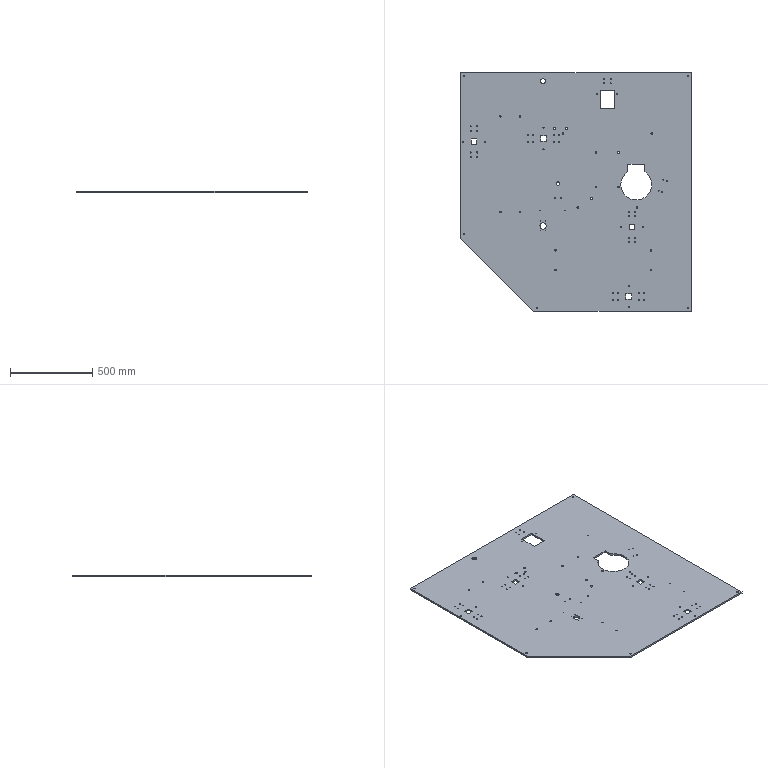Part | 1 solid | 203 faces | box 1400 x 1450 x 10 mm | volume 18802192 mm3 | cylinder 173 | plane 30 | commonest cylinder face diameters 6.8 x96 8.6 x34 3.3 x8 6 x8 10.2 x8 13 x6